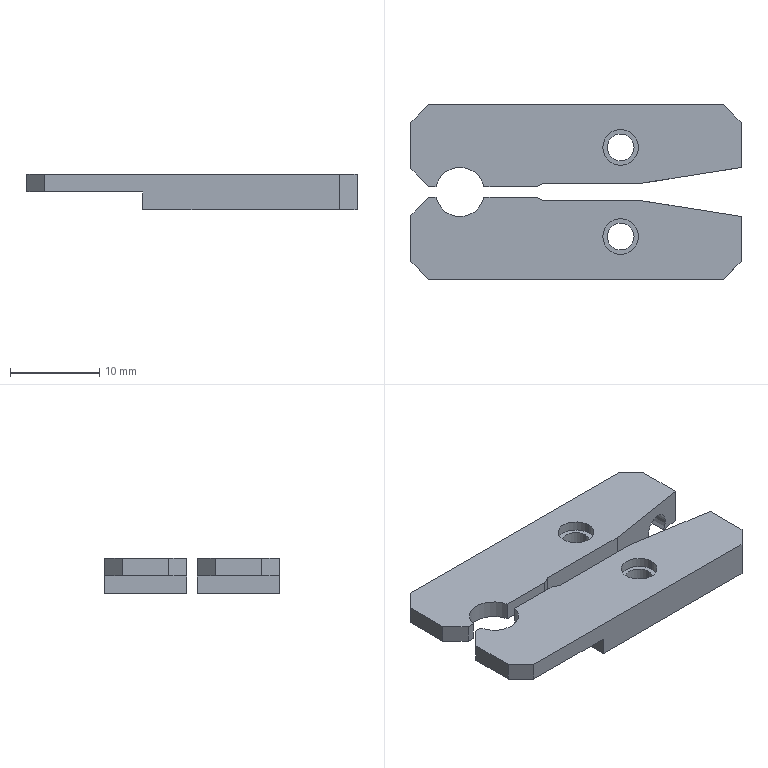Part | STEP file | BU-B03#260 | 2 solids | 49 faces | box 37 x 19.6 x 4 mm | volume 1912 mm3 | plane 32 | cylinder 13 | cone 4 | commonest cylinder face diameters 3 x4 4 x4 3.2 x3 5.5 x2